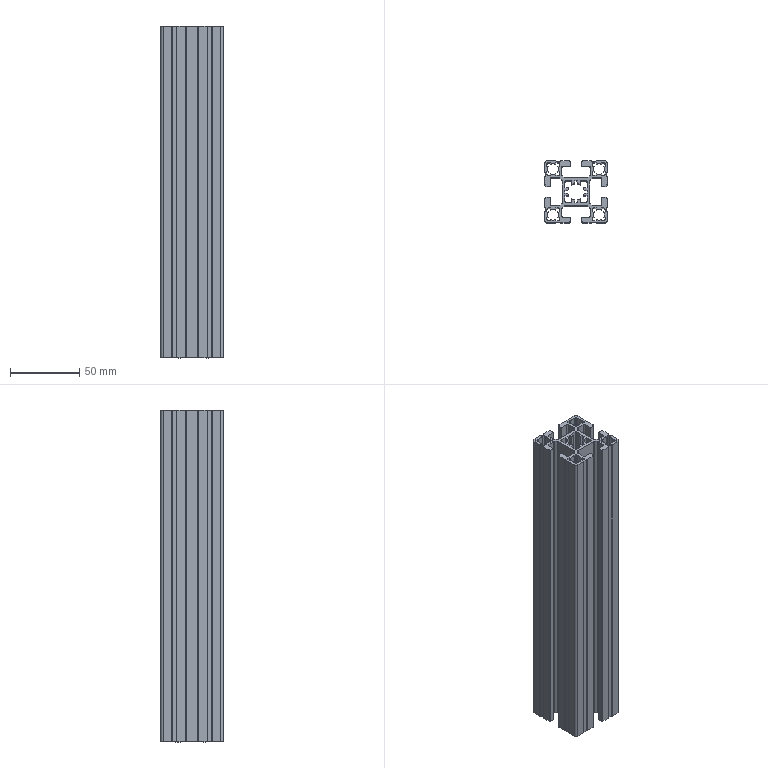Part | STEP file | 4545-240 Al (tri-LED mount) | 1 solid | 262 faces | box 45 x 45 x 240 mm | volume 166523 mm3 | plane 186 | cylinder 76 | commonest cylinder face diameters 2 x44 8 x20 12 x8 4 x4